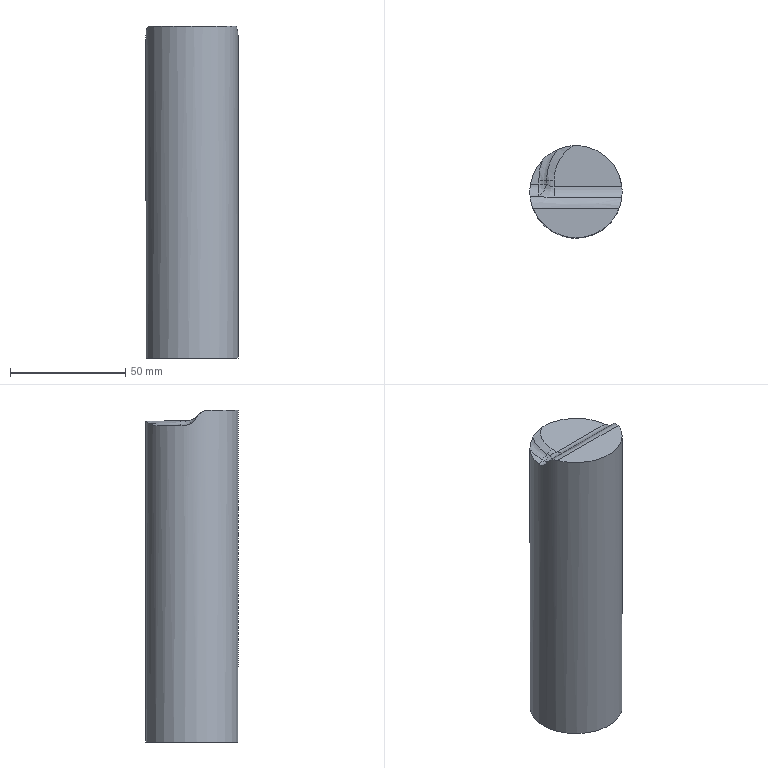Part | NX | features solid 2 | 1 solid | 14 faces | volume 177258 mm3 | spline 12 | cylinder 1 | plane 1 | commonest cylinder face diameters 40 x1
STEP:
#1=CARTESIAN_POINT('',(-644.903,-1.965,-10.409));
#2=VERTEX_POINT('',#1);
#3=CARTESIAN_POINT('',(-643.632,-7.27,-7.114));
#4=VERTEX_POINT('',#3);
#5=CARTESIAN_POINT('',(-644.903,-1.965,-10.409));
#6=CARTESIAN_POINT('',(-644.853,-2.474,-9.401));
#7=CARTESIAN_POINT('',(-644.661,-4.052,-7.717));
#8=CARTESIAN_POINT('',(-644.043,-6.217,-7.123));
#9=CARTESIAN_POINT('',(-643.632,-7.27,-7.114));
#10=B_SPLINE_CURVE_WITH_KNOTS('',3,(#5,#6,#7,#8,#9),.UNSPECIFIED.,.F.,.F.,(4,1,4),(0.,0.003343,0.006685),.UNSPECIFIED.);
#11=EDGE_CURVE('',#2,#4,#10,.T.);
#12=ORIENTED_EDGE('',*,*,#11,.F.);
#13=CARTESIAN_POINT('',(-644.719,3.34,-13.705));
#14=VERTEX_POINT('',#13);
#15=CARTESIAN_POINT('',(-644.719,3.34,-13.705));
#16=CARTESIAN_POINT('',(-645.089,1.157,-13.686));
#17=CARTESIAN_POINT('',(-645.002,-0.9681,-12.383));
#18=CARTESIAN_POINT('',(-644.903,-1.965,-10.409));
#19=B_SPLINE_CURVE_WITH_KNOTS('',3,(#15,#16,#17,#18),.UNSPECIFIED.,.F.,.F.,(4,4),(0.,0.006548),.UNSPECIFIED.);
#20=EDGE_CURVE('',#14,#2,#19,.T.);
#21=ORIENTED_EDGE('',*,*,#20,.F.);
#22=CARTESIAN_POINT('',(-639.509,13.765,-13.794));
#23=VERTEX_POINT('',#22);
#24=CARTESIAN_POINT('',(-639.509,13.765,-13.794));
#25=CARTESIAN_POINT('',(-642.206,10.923,-13.769));
#26=CARTESIAN_POINT('',(-644.056,7.257,-13.738));
#27=CARTESIAN_POINT('',(-644.719,3.34,-13.705));
#28=B_SPLINE_CURVE_WITH_KNOTS('',3,(#24,#25,#26,#27),.UNSPECIFIED.,.F.,.F.,(4,4),(0.04409,0.05584),.UNSPECIFIED.);
#29=EDGE_CURVE('',#23,#14,#28,.T.);
#30=ORIENTED_EDGE('',*,*,#29,.F.);
#31=CARTESIAN_POINT('',(-633.083,18.294,-12.832));
#32=VERTEX_POINT('',#31);
#33=CARTESIAN_POINT('',(-633.083,18.294,-12.832));
#34=CARTESIAN_POINT('',(-635.427,17.258,-13.593));
#35=CARTESIAN_POINT('',(-637.67,15.704,-13.81));
#36=CARTESIAN_POINT('',(-639.509,13.766,-13.794));
#37=B_SPLINE_CURVE_WITH_KNOTS('',3,(#33,#34,#35,#36),.UNSPECIFIED.,.F.,.F.,(4,4),(0.,0.00799),.UNSPECIFIED.);
#38=EDGE_CURVE('',#32,#23,#37,.T.);
#39=ORIENTED_EDGE('',*,*,#38,.F.);
#40=CARTESIAN_POINT('',(-626.243,19.961,-11.846));
#41=VERTEX_POINT('',#40);
#42=CARTESIAN_POINT('',(-626.24,19.962,-11.846));
#43=CARTESIAN_POINT('',(-628.632,19.813,-11.845));
#44=CARTESIAN_POINT('',(-630.98,19.223,-12.15));
#45=CARTESIAN_POINT('',(-633.083,18.294,-12.832));
#46=B_SPLINE_CURVE_WITH_KNOTS('',3,(#42,#43,#44,#45),.UNSPECIFIED.,.F.,.F.,(4,4),(0.,0.007178),.UNSPECIFIED.);
#47=EDGE_CURVE('',#41,#32,#46,.T.);
#48=ORIENTED_EDGE('',*,*,#47,.F.);
#49=CARTESIAN_POINT('',(-605.106,2.059,-11.694));
#50=VERTEX_POINT('',#49);
#51=CARTESIAN_POINT('',(-605.106,2.059,-11.694));
#52=CARTESIAN_POINT('',(-605.371,4.62,-11.715));
#53=CARTESIAN_POINT('',(-606.877,9.562,-11.758));
#54=CARTESIAN_POINT('',(-611.763,15.646,-11.81));
#55=CARTESIAN_POINT('',(-618.55,19.453,-11.842));
#56=CARTESIAN_POINT('',(-623.713,20.119,-11.848));
#57=CARTESIAN_POINT('',(-626.247,19.961,-11.846));
#58=B_SPLINE_CURVE_WITH_KNOTS('',3,(#51,#52,#53,#54,#55,#56,#57),.UNSPECIFIED.,.F.,.F.,(4,1,1,1,4),(0.,0.007614,0.01523,0.02284,0.03046),.UNSPECIFIED.);
#59=EDGE_CURVE('',#50,#41,#58,.T.);
#60=ORIENTED_EDGE('',*,*,#59,.F.);
#61=CARTESIAN_POINT('',(-605.17,-2.605,-9.404));
#62=VERTEX_POINT('',#61);
#63=CARTESIAN_POINT('',(-605.17,-2.605,-9.404));
#64=CARTESIAN_POINT('',(-605.024,-1.49,-10.821));
#65=CARTESIAN_POINT('',(-604.92,0.2592,-11.678));
#66=CARTESIAN_POINT('',(-605.106,2.059,-11.694));
#67=B_SPLINE_CURVE_WITH_KNOTS('',3,(#63,#64,#65,#66),.UNSPECIFIED.,.F.,.F.,(4,4),(0.,0.005391),.UNSPECIFIED.);
#68=EDGE_CURVE('',#62,#50,#67,.T.);
#69=ORIENTED_EDGE('',*,*,#68,.F.);
#70=CARTESIAN_POINT('',(-606.368,-7.27,-7.114));
#71=VERTEX_POINT('',#70);
#72=CARTESIAN_POINT('',(-606.368,-7.27,-7.114));
#73=CARTESIAN_POINT('',(-605.692,-5.537,-7.129));
#74=CARTESIAN_POINT('',(-605.319,-3.738,-7.963));
#75=CARTESIAN_POINT('',(-605.17,-2.605,-9.404));
#76=B_SPLINE_CURVE_WITH_KNOTS('',3,(#72,#73,#74,#75),.UNSPECIFIED.,.F.,.F.,(4,4),(0.,0.005504),.UNSPECIFIED.);
#77=EDGE_CURVE('',#71,#62,#76,.T.);
#78=ORIENTED_EDGE('',*,*,#77,.F.);
#79=CARTESIAN_POINT('',(-643.632,-7.27,-7.114));
#80=CARTESIAN_POINT('',(-642.165,-11.029,-7.082));
#81=CARTESIAN_POINT('',(-636.992,-17.511,-7.026));
#82=CARTESIAN_POINT('',(-624.988,-21.24,-6.994));
#83=CARTESIAN_POINT('',(-615.012,-18.146,-7.021));
#84=CARTESIAN_POINT('',(-609.089,-12.601,-7.068));
#85=CARTESIAN_POINT('',(-607.101,-9.149,-7.098));
#86=CARTESIAN_POINT('',(-606.368,-7.27,-7.114));
#87=B_SPLINE_CURVE_WITH_KNOTS('',3,(#79,#80,#81,#82,#83,#84,#85,#86),.UNSPECIFIED.,.F.,.F.,(4,1,1,1,1,4),(0.,0.01194,0.02387,0.03581,0.04177,0.04774),.UNSPECIFIED.);
#88=EDGE_CURVE('',#4,#71,#87,.T.);
#89=ORIENTED_EDGE('',*,*,#88,.F.);
#90=EDGE_LOOP('',(#12,#21,#30,#39,#48,#60,#69,#78,#89));
#91=FACE_BOUND('',#90,.T.);
#92=CARTESIAN_POINT('',(-605.,0.,-151.));
#93=VERTEX_POINT('',#92);
#94=CARTESIAN_POINT('',(-625.,0.,-151.));
#95=DIRECTION('',(0.,0.,1.));
#96=DIRECTION('',(1.,0.,0.));
#97=AXIS2_PLACEMENT_3D('',#94,#95,#96);
#98=CIRCLE('',#97,20.);
#99=EDGE_CURVE('',#93,#93,#98,.F.);
#100=ORIENTED_EDGE('',*,*,#99,.F.);
#101=EDGE_LOOP('',(#100));
#102=FACE_BOUND('',#101,.T.);
#103=CARTESIAN_POINT('',(-625.,0.,40.));
#104=DIRECTION('',(0.,0.,-1.));
#105=DIRECTION('',(-1.,0.,0.));
#106=AXIS2_PLACEMENT_3D('',#103,#104,#105);
#107=CYLINDRICAL_SURFACE('',#106,20.);
#108=ADVANCED_FACE('',(#91,#102),#107,.T.);
#109=ORIENTED_EDGE('',*,*,#99,.T.);
#110=EDGE_LOOP('',(#109));
#111=FACE_BOUND('',#110,.T.);
#112=CARTESIAN_POINT('',(-615.,0.,-151.));
#113=DIRECTION('',(0.,0.,1.));
#114=DIRECTION('',(1.,0.,0.));
#115=AXIS2_PLACEMENT_3D('',#112,#113,#114);
#116=PLANE('',#115);
#117=ADVANCED_FACE('',(#111),#116,.F.);
#118=ORIENTED_EDGE('',*,*,#29,.T.);
#119=CARTESIAN_POINT('',(-641.148,3.34,-13.705));
#120=VERTEX_POINT('',#119);
#121=CARTESIAN_POINT('',(-641.148,3.34,-13.705));
#122=CARTESIAN_POINT('',(-647.,3.34,-13.705));
#123=(BOUNDED_CURVE()B_SPLINE_CURVE(1,(#121,#122),.UNSPECIFIED.,.F.,.F.)B_SPLINE_CURVE_WITH_KNOTS((2,2),(0.,1.),.PIECEWISE_BEZIER_KNOTS.)CURVE()GEOMETRIC_REPRESENTATION_ITEM()RATIONAL_B_SPLINE_CURVE((1.,1.))REPRESENTATION_ITEM(''));
#124=EDGE_CURVE('',#14,#120,#123,.F.);
#125=ORIENTED_EDGE('',*,*,#124,.T.);
#126=CARTESIAN_POINT('',(-641.148,4.988,-13.719));
#127=VERTEX_POINT('',#126);
#128=CARTESIAN_POINT('',(-641.148,3.34,-13.705));
#129=CARTESIAN_POINT('',(-641.148,3.889,-13.709));
#130=CARTESIAN_POINT('',(-641.148,4.438,-13.714));
#131=CARTESIAN_POINT('',(-641.148,4.988,-13.719));
#132=B_SPLINE_CURVE_WITH_KNOTS('',3,(#128,#129,#130,#131),.UNSPECIFIED.,.F.,.F.,(4,4),(0.,1.),.UNSPECIFIED.);
#133=EDGE_CURVE('',#120,#127,#132,.T.);
#134=ORIENTED_EDGE('',*,*,#133,.T.);
#135=CARTESIAN_POINT('',(-641.148,4.988,-13.719));
#136=CARTESIAN_POINT('',(-641.148,8.023,-13.744));
#137=CARTESIAN_POINT('',(-640.602,10.949,-13.769));
#138=CARTESIAN_POINT('',(-639.509,13.765,-13.794));
#139=B_SPLINE_CURVE_WITH_KNOTS('',3,(#135,#136,#137,#138),.UNSPECIFIED.,.F.,.F.,(4,4),(0.,0.2363),.UNSPECIFIED.);
#140=EDGE_CURVE('',#127,#23,#139,.T.);
#141=ORIENTED_EDGE('',*,*,#140,.T.);
#142=EDGE_LOOP('',(#118,#125,#134,#141));
#143=FACE_BOUND('',#142,.T.);
#144=CARTESIAN_POINT('',(-639.478,13.828,-13.794));
#145=CARTESIAN_POINT('',(-644.75,13.828,-13.794));
#146=CARTESIAN_POINT('',(-639.478,3.34,-13.705));
#147=CARTESIAN_POINT('',(-644.75,3.34,-13.705));
#148=B_SPLINE_SURFACE_WITH_KNOTS('',1,1,((#144,#145),(#146,#147)),.PLANE_SURF.,.F.,.F.,.F.,(2,2),(2,2),(0.7723,1.),(0.9535,0.9861),.PIECEWISE_BEZIER_KNOTS.);
#149=ADVANCED_FACE('',(#143),#148,.F.);
#150=ORIENTED_EDGE('',*,*,#38,.T.);
#151=ORIENTED_EDGE('',*,*,#140,.F.);
#152=CARTESIAN_POINT('',(-637.831,4.996,-12.719));
#153=VERTEX_POINT('',#152);
#154=CARTESIAN_POINT('',(-637.831,4.996,-12.719));
#155=CARTESIAN_POINT('',(-638.807,4.991,-13.366));
#156=CARTESIAN_POINT('',(-639.977,4.988,-13.719));
#157=CARTESIAN_POINT('',(-641.148,4.988,-13.719));
#158=B_SPLINE_CURVE_WITH_KNOTS('',3,(#154,#155,#156,#157),.UNSPECIFIED.,.F.,.F.,(4,4),(0.,1.),.UNSPECIFIED.);
#159=EDGE_CURVE('',#127,#153,#158,.F.);
#160=ORIENTED_EDGE('',*,*,#159,.T.);
#161=CARTESIAN_POINT('',(-633.083,18.294,-12.832));
#162=CARTESIAN_POINT('',(-636.122,14.585,-12.8));
#163=CARTESIAN_POINT('',(-637.831,9.804,-12.76));
#164=CARTESIAN_POINT('',(-637.831,4.996,-12.719));
#165=B_SPLINE_CURVE_WITH_KNOTS('',3,(#161,#162,#163,#164),.UNSPECIFIED.,.F.,.F.,(4,4),(0.5612,1.),.UNSPECIFIED.);
#166=EDGE_CURVE('',#153,#32,#165,.F.);
#167=ORIENTED_EDGE('',*,*,#166,.T.);
#168=EDGE_LOOP('',(#150,#151,#160,#167));
#169=FACE_BOUND('',#168,.T.);
#170=CARTESIAN_POINT('',(-641.148,4.988,-13.719));
#171=CARTESIAN_POINT('',(-640.445,4.988,-13.719));
#172=CARTESIAN_POINT('',(-639.742,4.988,-13.616));
#173=CARTESIAN_POINT('',(-639.06,4.99,-13.41));
#174=CARTESIAN_POINT('',(-638.417,4.993,-13.107));
#175=CARTESIAN_POINT('',(-637.831,4.996,-12.719));
#176=CARTESIAN_POINT('',(-641.148,5.525,-13.723));
#177=CARTESIAN_POINT('',(-640.445,5.509,-13.723));
#178=CARTESIAN_POINT('',(-639.742,5.495,-13.62));
#179=CARTESIAN_POINT('',(-639.06,5.481,-13.414));
#180=CARTESIAN_POINT('',(-638.417,5.47,-13.111));
#181=CARTESIAN_POINT('',(-637.831,5.46,-12.723));
#182=CARTESIAN_POINT('',(-641.133,6.068,-13.728));
#183=CARTESIAN_POINT('',(-640.431,6.036,-13.728));
#184=CARTESIAN_POINT('',(-639.728,6.006,-13.624));
#185=CARTESIAN_POINT('',(-639.046,5.977,-13.418));
#186=CARTESIAN_POINT('',(-638.404,5.951,-13.115));
#187=CARTESIAN_POINT('',(-637.818,5.929,-12.727));
#188=CARTESIAN_POINT('',(-641.103,6.599,-13.732));
#189=CARTESIAN_POINT('',(-640.402,6.552,-13.732));
#190=CARTESIAN_POINT('',(-639.7,6.507,-13.629));
#191=CARTESIAN_POINT('',(-639.019,6.463,-13.422));
#192=CARTESIAN_POINT('',(-638.377,6.423,-13.119));
#193=CARTESIAN_POINT('',(-637.793,6.388,-12.731));
#194=CARTESIAN_POINT('',(-641.015,7.671,-13.741));
#195=CARTESIAN_POINT('',(-640.316,7.594,-13.741));
#196=CARTESIAN_POINT('',(-639.617,7.517,-13.637));
#197=CARTESIAN_POINT('',(-638.938,7.444,-13.431));
#198=CARTESIAN_POINT('',(-638.299,7.375,-13.127));
#199=CARTESIAN_POINT('',(-637.716,7.314,-12.738));
#200=CARTESIAN_POINT('',(-640.867,8.733,-13.751));
#201=CARTESIAN_POINT('',(-640.172,8.625,-13.75));
#202=CARTESIAN_POINT('',(-639.477,8.517,-13.646));
#203=CARTESIAN_POINT('',(-638.803,8.414,-13.439));
#204=CARTESIAN_POINT('',(-638.167,8.318,-13.135));
#205=CARTESIAN_POINT('',(-637.589,8.231,-12.746));
#206=CARTESIAN_POINT('',(-640.778,9.264,-13.755));
#207=CARTESIAN_POINT('',(-640.086,9.14,-13.754));
#208=CARTESIAN_POINT('',(-639.394,9.018,-13.65));
#209=CARTESIAN_POINT('',(-638.722,8.899,-13.443));
#210=CARTESIAN_POINT('',(-638.089,8.789,-13.14));
#211=CARTESIAN_POINT('',(-637.512,8.689,-12.75));
#212=CARTESIAN_POINT('',(-640.469,10.845,-13.769));
#213=CARTESIAN_POINT('',(-639.786,10.675,-13.767));
#214=CARTESIAN_POINT('',(-639.103,10.507,-13.663));
#215=CARTESIAN_POINT('',(-638.439,10.344,-13.456));
#216=CARTESIAN_POINT('',(-637.814,10.192,-13.151));
#217=CARTESIAN_POINT('',(-637.245,10.055,-12.762));
#218=CARTESIAN_POINT('',(-640.03,12.396,-13.782));
#219=CARTESIAN_POINT('',(-639.359,12.182,-13.78));
#220=CARTESIAN_POINT('',(-638.689,11.969,-13.675));
#221=CARTESIAN_POINT('',(-638.037,11.763,-13.468));
#222=CARTESIAN_POINT('',(-637.424,11.57,-13.163));
#223=CARTESIAN_POINT('',(-636.866,11.395,-12.773));
#224=CARTESIAN_POINT('',(-639.68,13.413,-13.791));
#225=CARTESIAN_POINT('',(-639.02,13.17,-13.788));
#226=CARTESIAN_POINT('',(-638.359,12.927,-13.683));
#227=CARTESIAN_POINT('',(-637.718,12.692,-13.476));
#228=CARTESIAN_POINT('',(-637.114,12.472,-13.171));
#229=CARTESIAN_POINT('',(-636.564,12.273,-12.781));
#230=CARTESIAN_POINT('',(-638.819,15.53,-13.809));
#231=CARTESIAN_POINT('',(-638.183,15.225,-13.806));
#232=CARTESIAN_POINT('',(-637.548,14.921,-13.7));
#233=CARTESIAN_POINT('',(-636.931,14.627,-13.492));
#234=CARTESIAN_POINT('',(-636.35,14.351,-13.187));
#235=CARTESIAN_POINT('',(-635.82,14.101,-12.796));
#236=CARTESIAN_POINT('',(-637.715,17.532,-13.826));
#237=CARTESIAN_POINT('',(-637.112,17.169,-13.823));
#238=CARTESIAN_POINT('',(-636.508,16.807,-13.717));
#239=CARTESIAN_POINT('',(-635.922,16.457,-13.508));
#240=CARTESIAN_POINT('',(-635.37,16.128,-13.202));
#241=CARTESIAN_POINT('',(-634.867,15.829,-12.811));
#242=CARTESIAN_POINT('',(-637.066,18.554,-13.834));
#243=CARTESIAN_POINT('',(-636.481,18.162,-13.831));
#244=CARTESIAN_POINT('',(-635.896,17.771,-13.725));
#245=CARTESIAN_POINT('',(-635.328,17.391,-13.516));
#246=CARTESIAN_POINT('',(-634.794,17.035,-13.21));
#247=CARTESIAN_POINT('',(-634.306,16.712,-12.819));
#248=CARTESIAN_POINT('',(-636.354,19.534,-13.843));
#249=CARTESIAN_POINT('',(-635.79,19.113,-13.839));
#250=CARTESIAN_POINT('',(-635.226,18.693,-13.733));
#251=CARTESIAN_POINT('',(-634.678,18.286,-13.523));
#252=CARTESIAN_POINT('',(-634.162,17.904,-13.217));
#253=CARTESIAN_POINT('',(-633.692,17.557,-12.826));
#254=CARTESIAN_POINT('',(-635.584,20.465,-13.851));
#255=CARTESIAN_POINT('',(-635.042,20.017,-13.847));
#256=CARTESIAN_POINT('',(-634.501,19.57,-13.74));
#257=CARTESIAN_POINT('',(-633.974,19.137,-13.531));
#258=CARTESIAN_POINT('',(-633.479,18.731,-13.224));
#259=CARTESIAN_POINT('',(-633.028,18.361,-12.833));
#260=B_SPLINE_SURFACE_WITH_KNOTS('',5,5,((#170,#171,#172,#173,#174,#175),(#176,#177,#178,#179,#180,#181),(#182,#183,#184,#185,#186,#187),(#188,#189,#190,#191,#192,#193),(#194,#195,#196,#197,#198,#199),(#200,#201,#202,#203,#204,#205),(#206,#207,#208,#209,#210,#211),(#212,#213,#214,#215,#216,#217),(#218,#219,#220,#221,#222,#223),(#224,#225,#226,#227,#228,#229),(#230,#231,#232,#233,#234,#235),(#236,#237,#238,#239,#240,#241),(#242,#243,#244,#245,#246,#247),(#248,#249,#250,#251,#252,#253),(#254,#255,#256,#257,#258,#259)),.UNSPECIFIED.,.F.,.F.,.F.,(6,3,3,3,6),(6,6),(0.,0.0706,0.1412,0.2824,0.4414),(0.,1.),.UNSPECIFIED.);
#261=ADVANCED_FACE('',(#169),#260,.F.);
#262=CARTESIAN_POINT('',(-637.831,3.349,-12.705));
#263=VERTEX_POINT('',#262);
#264=CARTESIAN_POINT('',(-637.831,3.349,-12.705));
#265=CARTESIAN_POINT('',(-638.794,3.343,-13.343));
#266=CARTESIAN_POINT('',(-639.993,3.34,-13.705));
#267=CARTESIAN_POINT('',(-641.148,3.34,-13.705));
#268=B_SPLINE_CURVE_WITH_KNOTS('',3,(#264,#265,#266,#267),.UNSPECIFIED.,.F.,.F.,(4,4),(0.,1.),.UNSPECIFIED.);
#269=EDGE_CURVE('',#120,#263,#268,.F.);
#270=ORIENTED_EDGE('',*,*,#269,.T.);
#271=CARTESIAN_POINT('',(-637.831,4.996,-12.719));
#272=CARTESIAN_POINT('',(-637.831,4.447,-12.714));
#273=CARTESIAN_POINT('',(-637.831,3.898,-12.709));
#274=CARTESIAN_POINT('',(-637.831,3.349,-12.705));
#275=B_SPLINE_CURVE_WITH_KNOTS('',3,(#271,#272,#273,#274),.UNSPECIFIED.,.F.,.F.,(4,4),(0.,1.),.UNSPECIFIED.);
#276=EDGE_CURVE('',#153,#263,#275,.T.);
#277=ORIENTED_EDGE('',*,*,#276,.F.);
#278=ORIENTED_EDGE('',*,*,#159,.F.);
#279=ORIENTED_EDGE('',*,*,#133,.F.);
#280=EDGE_LOOP('',(#270,#277,#278,#279));
#281=FACE_BOUND('',#280,.T.);
#282=CARTESIAN_POINT('',(-637.831,3.349,-12.705));
#283=CARTESIAN_POINT('',(-637.831,4.996,-12.719));
#284=CARTESIAN_POINT('',(-638.822,3.343,-13.361));
#285=CARTESIAN_POINT('',(-638.822,4.99,-13.376));
#286=CARTESIAN_POINT('',(-639.96,3.34,-13.705));
#287=CARTESIAN_POINT('',(-639.96,4.988,-13.719));
#288=CARTESIAN_POINT('',(-641.148,3.34,-13.705));
#289=CARTESIAN_POINT('',(-641.148,4.988,-13.719));
#290=(BOUNDED_SURFACE()B_SPLINE_SURFACE(3,1,((#282,#283),(#284,#285),(#286,#287),(#288,#289)),.CYLINDRICAL_SURF.,.F.,.F.,.F.)B_SPLINE_SURFACE_WITH_KNOTS((4,4),(2,2),(0.,1.),(0.,1.),.PIECEWISE_BEZIER_KNOTS.)GEOMETRIC_REPRESENTATION_ITEM()RATIONAL_B_SPLINE_SURFACE(((1.,1.),(0.9716,0.9716),(0.9716,0.9716),(1.,1.)))REPRESENTATION_ITEM('')SURFACE());
#291=ADVANCED_FACE('',(#281),#290,.F.);
#292=ORIENTED_EDGE('',*,*,#20,.T.);
#293=CARTESIAN_POINT('',(-641.148,-1.965,-10.409));
#294=VERTEX_POINT('',#293);
#295=CARTESIAN_POINT('',(-641.148,-1.965,-10.409));
#296=CARTESIAN_POINT('',(-642.4,-1.965,-10.409));
#297=CARTESIAN_POINT('',(-643.651,-1.965,-10.409));
#298=CARTESIAN_POINT('',(-644.903,-1.965,-10.409));
#299=B_SPLINE_CURVE_WITH_KNOTS('',3,(#295,#296,#297,#298),.UNSPECIFIED.,.F.,.F.,(4,4),(0.,0.6417),.UNSPECIFIED.);
#300=EDGE_CURVE('',#294,#2,#299,.T.);
#301=ORIENTED_EDGE('',*,*,#300,.F.);
#302=CARTESIAN_POINT('',(-641.148,3.34,-13.705));
#303=CARTESIAN_POINT('',(-641.148,2.299,-13.696));
#304=CARTESIAN_POINT('',(-641.148,0.04839,-13.086));
#305=CARTESIAN_POINT('',(-641.148,-1.496,-11.338));
#306=CARTESIAN_POINT('',(-641.148,-1.965,-10.409));
#307=B_SPLINE_CURVE_WITH_KNOTS('',3,(#302,#303,#304,#305,#306),.UNSPECIFIED.,.F.,.F.,(4,1,4),(0.,0.5,1.),.UNSPECIFIED.);
#308=EDGE_CURVE('',#120,#294,#307,.T.);
#309=ORIENTED_EDGE('',*,*,#308,.F.);
#310=ORIENTED_EDGE('',*,*,#124,.F.);
#311=EDGE_LOOP('',(#292,#301,#309,#310));
#312=FACE_BOUND('',#311,.T.);
#313=CARTESIAN_POINT('',(-641.148,3.34,-13.705));
#314=CARTESIAN_POINT('',(-645.028,3.34,-13.705));
#315=CARTESIAN_POINT('',(-641.148,1.034,-13.685));
#316=CARTESIAN_POINT('',(-645.028,1.034,-13.685));
#317=CARTESIAN_POINT('',(-641.148,-0.9252,-12.468));
#318=CARTESIAN_POINT('',(-645.028,-0.9252,-12.468));
#319=CARTESIAN_POINT('',(-641.148,-1.965,-10.409));
#320=CARTESIAN_POINT('',(-645.028,-1.965,-10.409));
#321=(BOUNDED_SURFACE()B_SPLINE_SURFACE(3,1,((#313,#314),(#315,#316),(#317,#318),(#319,#320)),.CYLINDRICAL_SURF.,.F.,.F.,.F.)B_SPLINE_SURFACE_WITH_KNOTS((4,4),(2,2),(0.,1.),(0.,0.6631),.PIECEWISE_BEZIER_KNOTS.)GEOMETRIC_REPRESENTATION_ITEM()RATIONAL_B_SPLINE_SURFACE(((1.,1.),(0.9026,0.9026),(0.9026,0.9026),(1.,1.)))REPRESENTATION_ITEM('')SURFACE());
#322=ADVANCED_FACE('',(#312),#321,.F.);
#323=ORIENTED_EDGE('',*,*,#47,.T.);
#324=ORIENTED_EDGE('',*,*,#166,.F.);
#325=CARTESIAN_POINT('',(-634.515,5.005,-11.719));
#326=VERTEX_POINT('',#325);
#327=CARTESIAN_POINT('',(-634.515,5.005,-11.719));
#328=CARTESIAN_POINT('',(-635.686,5.005,-11.719));
#329=CARTESIAN_POINT('',(-636.855,5.002,-12.071));
#330=CARTESIAN_POINT('',(-637.831,4.996,-12.719));
#331=B_SPLINE_CURVE_WITH_KNOTS('',3,(#327,#328,#329,#330),.UNSPECIFIED.,.F.,.F.,(4,4),(0.,1.),.UNSPECIFIED.);
#332=EDGE_CURVE('',#326,#153,#331,.T.);
#333=ORIENTED_EDGE('',*,*,#332,.F.);
#334=CARTESIAN_POINT('',(-626.243,19.96,-11.846));
#335=CARTESIAN_POINT('',(-628.759,18.388,-11.833));
#336=CARTESIAN_POINT('',(-632.976,13.938,-11.795));
#337=CARTESIAN_POINT('',(-634.515,7.986,-11.744));
#338=CARTESIAN_POINT('',(-634.515,5.005,-11.719));
#339=B_SPLINE_CURVE_WITH_KNOTS('',3,(#334,#335,#336,#337,#338),.UNSPECIFIED.,.F.,.F.,(4,1,4),(0.3537,0.6768,1.),.UNSPECIFIED.);
#340=EDGE_CURVE('',#326,#41,#339,.F.);
#341=ORIENTED_EDGE('',*,*,#340,.T.);
#342=EDGE_LOOP('',(#323,#324,#333,#341));
#343=FACE_BOUND('',#342,.T.);
#344=CARTESIAN_POINT('',(-626.149,20.018,-11.847));
#345=CARTESIAN_POINT('',(-626.518,20.616,-11.852));
#346=CARTESIAN_POINT('',(-626.886,21.214,-11.96));
#347=CARTESIAN_POINT('',(-627.244,21.793,-12.171));
#348=CARTESIAN_POINT('',(-627.581,22.338,-12.478));
#349=CARTESIAN_POINT('',(-627.888,22.833,-12.871));
#350=CARTESIAN_POINT('',(-626.484,19.812,-11.845));
#351=CARTESIAN_POINT('',(-626.866,20.402,-11.85));
#352=CARTESIAN_POINT('',(-627.248,20.991,-11.958));
#353=CARTESIAN_POINT('',(-627.619,21.563,-12.169));
#354=CARTESIAN_POINT('',(-627.968,22.1,-12.476));
#355=CARTESIAN_POINT('',(-628.286,22.588,-12.869));
#356=CARTESIAN_POINT('',(-626.812,19.597,-11.843));
#357=CARTESIAN_POINT('',(-627.207,20.178,-11.848));
#358=CARTESIAN_POINT('',(-627.602,20.759,-11.956));
#359=CARTESIAN_POINT('',(-627.986,21.322,-12.167));
#360=CARTESIAN_POINT('',(-628.348,21.851,-12.474));
#361=CARTESIAN_POINT('',(-628.677,22.332,-12.867));
#362=CARTESIAN_POINT('',(-627.135,19.372,-11.841));
#363=CARTESIAN_POINT('',(-627.543,19.945,-11.846));
#364=CARTESIAN_POINT('',(-627.951,20.516,-11.954));
#365=CARTESIAN_POINT('',(-628.347,21.071,-12.165));
#366=CARTESIAN_POINT('',(-628.72,21.591,-12.472));
#367=CARTESIAN_POINT('',(-629.06,22.065,-12.864));
#368=CARTESIAN_POINT('',(-630.018,17.243,-11.823));
#369=CARTESIAN_POINT('',(-630.542,17.73,-11.827));
#370=CARTESIAN_POINT('',(-631.066,18.216,-11.934));
#371=CARTESIAN_POINT('',(-631.574,18.687,-12.144));
#372=CARTESIAN_POINT('',(-632.053,19.13,-12.451));
#373=CARTESIAN_POINT('',(-632.49,19.533,-12.843));
#374=CARTESIAN_POINT('',(-632.34,14.391,-11.799));
#375=CARTESIAN_POINT('',(-632.956,14.764,-11.802));
#376=CARTESIAN_POINT('',(-633.572,15.136,-11.908));
#377=CARTESIAN_POINT('',(-634.171,15.496,-12.117));
#378=CARTESIAN_POINT('',(-634.735,15.835,-12.423));
#379=CARTESIAN_POINT('',(-635.249,16.142,-12.814));
#380=CARTESIAN_POINT('',(-633.79,11.411,-11.773));
#381=CARTESIAN_POINT('',(-634.464,11.666,-11.776));
#382=CARTESIAN_POINT('',(-635.138,11.92,-11.881));
#383=CARTESIAN_POINT('',(-635.793,12.166,-12.089));
#384=CARTESIAN_POINT('',(-636.409,12.396,-12.393));
#385=CARTESIAN_POINT('',(-636.971,12.605,-12.784));
#386=CARTESIAN_POINT('',(-634.515,8.21,-11.746));
#387=CARTESIAN_POINT('',(-635.218,8.337,-11.747));
#388=CARTESIAN_POINT('',(-635.92,8.463,-11.851));
#389=CARTESIAN_POINT('',(-636.603,8.584,-12.058));
#390=CARTESIAN_POINT('',(-637.246,8.698,-12.362));
#391=CARTESIAN_POINT('',(-637.831,8.8,-12.751));
#392=CARTESIAN_POINT('',(-634.515,5.005,-11.719));
#393=CARTESIAN_POINT('',(-635.218,5.005,-11.719));
#394=CARTESIAN_POINT('',(-635.92,5.004,-11.822));
#395=CARTESIAN_POINT('',(-636.603,5.002,-12.027));
#396=CARTESIAN_POINT('',(-637.246,4.999,-12.33));
#397=CARTESIAN_POINT('',(-637.831,4.996,-12.719));
#398=B_SPLINE_SURFACE_WITH_KNOTS('',5,5,((#344,#345,#346,#347,#348,#349),(#350,#351,#352,#353,#354,#355),(#356,#357,#358,#359,#360,#361),(#362,#363,#364,#365,#366,#367),(#368,#369,#370,#371,#372,#373),(#374,#375,#376,#377,#378,#379),(#380,#381,#382,#383,#384,#385),(#386,#387,#388,#389,#390,#391),(#392,#393,#394,#395,#396,#397)),.UNSPECIFIED.,.F.,.F.,.F.,(6,3,6),(6,6),(0.3497,0.421,1.),(0.,0.994),.UNSPECIFIED.);
#399=ADVANCED_FACE('',(#343),#398,.F.);
#400=CARTESIAN_POINT('',(-634.515,2.059,-11.694));
#401=VERTEX_POINT('',#400);
#402=CARTESIAN_POINT('',(-634.515,2.059,-11.694));
#403=CARTESIAN_POINT('',(-634.515,3.041,-11.702));
#404=CARTESIAN_POINT('',(-634.515,4.023,-11.71));
#405=CARTESIAN_POINT('',(-634.515,5.005,-11.719));
#406=B_SPLINE_CURVE_WITH_KNOTS('',3,(#402,#403,#404,#405),.UNSPECIFIED.,.F.,.F.,(4,4),(0.,1.),.UNSPECIFIED.);
#407=EDGE_CURVE('',#401,#326,#406,.T.);
#408=ORIENTED_EDGE('',*,*,#407,.T.);
#409=ORIENTED_EDGE('',*,*,#332,.T.);
#410=ORIENTED_EDGE('',*,*,#276,.T.);
#411=CARTESIAN_POINT('',(-637.831,3.349,-12.705));
#412=CARTESIAN_POINT('',(-637.491,3.118,-12.477));
#413=CARTESIAN_POINT('',(-637.023,2.834,-12.235));
#414=CARTESIAN_POINT('',(-636.498,2.559,-12.033));
#415=CARTESIAN_POINT('',(-636.275,2.45,-11.956));
#416=CARTESIAN_POINT('',(-635.774,2.258,-11.821));
#417=CARTESIAN_POINT('',(-635.212,2.11,-11.724));
#418=CARTESIAN_POINT('',(-634.784,2.059,-11.694));
#419=CARTESIAN_POINT('',(-634.515,2.059,-11.694));
#420=B_SPLINE_CURVE_WITH_KNOTS('',3,(#411,#412,#413,#414,#415,#416,#417,#418,#419),.UNSPECIFIED.,.F.,.F.,(4,1,1,1,1,1,4),(0.,0.25,0.375,0.5,0.625,0.75,1.),.UNSPECIFIED.);
#421=EDGE_CURVE('',#263,#401,#420,.T.);
#422=ORIENTED_EDGE('',*,*,#421,.T.);
#423=EDGE_LOOP('',(#408,#409,#410,#422));
#424=FACE_BOUND('',#423,.T.);
#425=CARTESIAN_POINT('',(-634.515,5.005,-11.719));
#426=CARTESIAN_POINT('',(-634.515,2.042,-11.693));
#427=CARTESIAN_POINT('',(-635.703,5.005,-11.719));
#428=CARTESIAN_POINT('',(-635.703,2.042,-11.693));
#429=CARTESIAN_POINT('',(-636.841,5.002,-12.062));
#430=CARTESIAN_POINT('',(-636.841,2.039,-12.036));
#431=CARTESIAN_POINT('',(-637.831,4.996,-12.719));
#432=CARTESIAN_POINT('',(-637.831,2.033,-12.693));
#433=(BOUNDED_SURFACE()B_SPLINE_SURFACE(3,1,((#425,#426),(#427,#428),(#429,#430),(#431,#432)),.CYLINDRICAL_SURF.,.F.,.F.,.F.)B_SPLINE_SURFACE_WITH_KNOTS((4,4),(2,2),(0.,1.),(0.08333,0.9167),.PIECEWISE_BEZIER_KNOTS.)GEOMETRIC_REPRESENTATION_ITEM()RATIONAL_B_SPLINE_SURFACE(((1.,1.),(0.9716,0.9716),(0.9716,0.9716),(1.,1.)))REPRESENTATION_ITEM('')SURFACE());
#434=ADVANCED_FACE('',(#424),#433,.T.);
#435=ORIENTED_EDGE('',*,*,#269,.F.);
#436=ORIENTED_EDGE('',*,*,#308,.T.);
#437=CARTESIAN_POINT('',(-637.831,3.349,-12.705));
#438=CARTESIAN_POINT('',(-637.945,2.867,-12.776));
#439=CARTESIAN_POINT('',(-638.183,2.089,-12.821));
#440=CARTESIAN_POINT('',(-638.623,1.1,-12.657));
#441=CARTESIAN_POINT('',(-638.898,0.5681,-12.509));
#442=CARTESIAN_POINT('',(-639.187,0.08387,-12.317));
#443=CARTESIAN_POINT('',(-639.272,-0.04024,-12.256));
#444=CARTESIAN_POINT('',(-639.51,-0.3857,-12.082));
#445=CARTESIAN_POINT('',(-640.003,-1.019,-11.678));
#446=CARTESIAN_POINT('',(-640.644,-1.662,-11.01));
#447=CARTESIAN_POINT('',(-641.148,-1.965,-10.409));
#448=B_SPLINE_CURVE_WITH_KNOTS('',3,(#437,#438,#439,#440,#441,#442,#443,#444,#445,#446,#447),.UNSPECIFIED.,.F.,.F.,(4,1,1,1,1,1,1,1,4),(0.,0.25,0.375,0.4375,0.5,0.5625,0.625,0.75,1.),.UNSPECIFIED.);
#449=EDGE_CURVE('',#294,#263,#448,.F.);
#450=ORIENTED_EDGE('',*,*,#449,.T.);
#451=EDGE_LOOP('',(#435,#436,#450));
#452=FACE_BOUND('',#451,.T.);
#453=CARTESIAN_POINT('',(-641.148,3.34,-13.705));
#454=CARTESIAN_POINT('',(-641.148,1.018,-13.685));
#455=CARTESIAN_POINT('',(-641.148,-0.9487,-12.453));
#456=CARTESIAN_POINT('',(-641.148,-1.982,-10.376));
#457=CARTESIAN_POINT('',(-639.952,3.34,-13.705));
#458=CARTESIAN_POINT('',(-639.952,1.018,-13.685));
#459=CARTESIAN_POINT('',(-639.952,-0.9487,-12.453));
#460=CARTESIAN_POINT('',(-639.952,-1.982,-10.376));
#461=CARTESIAN_POINT('',(-638.808,3.343,-13.357));
#462=CARTESIAN_POINT('',(-638.808,1.156,-13.339));
#463=CARTESIAN_POINT('',(-638.808,-0.6976,-12.178));
#464=CARTESIAN_POINT('',(-638.808,-1.671,-10.221));
#465=CARTESIAN_POINT('',(-637.814,3.349,-12.693));
#466=CARTESIAN_POINT('',(-637.814,1.418,-12.677));
#467=CARTESIAN_POINT('',(-637.814,-0.2171,-11.653));
#468=CARTESIAN_POINT('',(-637.814,-1.076,-9.925));
#469=(BOUNDED_SURFACE()B_SPLINE_SURFACE(3,3,((#453,#454,#455,#456),(#457,#458,#459,#460),(#461,#462,#463,#464),(#465,#466,#467,#468)),.SPHERICAL_SURF.,.F.,.F.,.F.)B_SPLINE_SURFACE_WITH_KNOTS((4,4),(4,4),(0.,0.9999),(0.08628,0.9189),.PIECEWISE_BEZIER_KNOTS.)GEOMETRIC_REPRESENTATION_ITEM()RATIONAL_B_SPLINE_SURFACE(((0.9675,0.8727,0.8733,0.9692),(0.9397,0.8476,0.8482,0.9414),(0.9397,0.8476,0.8482,0.9414),(0.9675,0.8727,0.8733,0.9692)))REPRESENTATION_ITEM('')SURFACE());
#470=ADVANCED_FACE('',(#452),#469,.F.);
#471=ORIENTED_EDGE('',*,*,#59,.T.);
#472=ORIENTED_EDGE('',*,*,#340,.F.);
#473=ORIENTED_EDGE('',*,*,#407,.F.);
#474=CARTESIAN_POINT('',(-605.106,2.059,-11.694));
#475=CARTESIAN_POINT('',(-614.909,2.059,-11.694));
#476=CARTESIAN_POINT('',(-624.712,2.059,-11.694));
#477=CARTESIAN_POINT('',(-634.515,2.059,-11.694));
#478=B_SPLINE_CURVE_WITH_KNOTS('',3,(#474,#475,#476,#477),.UNSPECIFIED.,.F.,.F.,(4,4),(0.5973,1.),.UNSPECIFIED.);
#479=EDGE_CURVE('',#401,#50,#478,.F.);
#480=ORIENTED_EDGE('',*,*,#479,.T.);
#481=EDGE_LOOP('',(#471,#472,#473,#480));
#482=FACE_BOUND('',#481,.T.);
#483=CARTESIAN_POINT('',(-604.93,20.144,-11.848));
#484=CARTESIAN_POINT('',(-634.515,20.144,-11.848));
#485=CARTESIAN_POINT('',(-604.93,2.059,-11.694));
#486=CARTESIAN_POINT('',(-634.515,2.059,-11.694));
#487=B_SPLINE_SURFACE_WITH_KNOTS('',1,1,((#483,#484),(#485,#486)),.PLANE_SURF.,.F.,.F.,.F.,(2,2),(2,2),(0.12,1.),(0.5949,1.),.PIECEWISE_BEZIER_KNOTS.);
#488=ADVANCED_FACE('',(#482),#487,.F.);
#489=CARTESIAN_POINT('',(-634.515,-2.605,-9.404));
#490=VERTEX_POINT('',#489);
#491=CARTESIAN_POINT('',(-634.515,-2.605,-9.404));
#492=CARTESIAN_POINT('',(-636.83,-2.605,-9.404));
#493=CARTESIAN_POINT('',(-639.111,-2.307,-9.731));
#494=CARTESIAN_POINT('',(-641.148,-1.965,-10.409));
#495=B_SPLINE_CURVE_WITH_KNOTS('',3,(#491,#492,#493,#494),.UNSPECIFIED.,.F.,.F.,(4,4),(0.,1.),.UNSPECIFIED.);
#496=EDGE_CURVE('',#490,#294,#495,.T.);
#497=ORIENTED_EDGE('',*,*,#496,.F.);
#498=CARTESIAN_POINT('',(-634.515,2.059,-11.694));
#499=CARTESIAN_POINT('',(-634.515,0.268,-11.678));
#500=CARTESIAN_POINT('',(-634.515,-1.498,-10.811));
#501=CARTESIAN_POINT('',(-634.515,-2.605,-9.404));
#502=B_SPLINE_CURVE_WITH_KNOTS('',3,(#498,#499,#500,#501),.UNSPECIFIED.,.F.,.F.,(4,4),(0.,1.),.UNSPECIFIED.);
#503=EDGE_CURVE('',#401,#490,#502,.T.);
#504=ORIENTED_EDGE('',*,*,#503,.F.);
#505=ORIENTED_EDGE('',*,*,#421,.F.);
#506=ORIENTED_EDGE('',*,*,#449,.F.);
#507=EDGE_LOOP('',(#497,#504,#505,#506));
#508=FACE_BOUND('',#507,.T.);
#509=CARTESIAN_POINT('',(-634.515,-2.605,-9.404));
#510=CARTESIAN_POINT('',(-634.515,-1.941,-10.248));
#511=CARTESIAN_POINT('',(-634.515,-1.087,-10.944));
#512=CARTESIAN_POINT('',(-634.515,-0.08822,-11.435));
#513=CARTESIAN_POINT('',(-634.515,0.9845,-11.684));
#514=CARTESIAN_POINT('',(-634.515,2.059,-11.694));
#515=CARTESIAN_POINT('',(-634.992,-2.605,-9.404));
#516=CARTESIAN_POINT('',(-634.937,-1.941,-10.248));
#517=CARTESIAN_POINT('',(-634.883,-1.087,-10.944));
#518=CARTESIAN_POINT('',(-634.832,-0.08822,-11.435));
#519=CARTESIAN_POINT('',(-634.788,0.9845,-11.684));
#520=CARTESIAN_POINT('',(-634.753,2.059,-11.694));
#521=CARTESIAN_POINT('',(-635.47,-2.596,-9.416));
#522=CARTESIAN_POINT('',(-635.36,-1.932,-10.263));
#523=CARTESIAN_POINT('',(-635.25,-1.078,-10.961));
#524=CARTESIAN_POINT('',(-635.148,-0.07651,-11.452));
#525=CARTESIAN_POINT('',(-635.061,0.9998,-11.7));
#526=CARTESIAN_POINT('',(-634.992,2.078,-11.706));
#527=CARTESIAN_POINT('',(-635.945,-2.577,-9.439));
#528=CARTESIAN_POINT('',(-635.781,-1.916,-10.293));
#529=CARTESIAN_POINT('',(-635.616,-1.06,-10.994));
#530=CARTESIAN_POINT('',(-635.463,-0.05309,-11.486));
#531=CARTESIAN_POINT('',(-635.332,1.03,-11.731));
#532=CARTESIAN_POINT('',(-635.23,2.116,-11.73));
#533=CARTESIAN_POINT('',(-637.321,-2.497,-9.544));
#534=CARTESIAN_POINT('',(-636.996,-1.847,-10.421));
#535=CARTESIAN_POINT('',(-636.67,-0.9835,-11.139));
#536=CARTESIAN_POINT('',(-636.368,0.04614,-11.633));
#537=CARTESIAN_POINT('',(-636.113,1.161,-11.864));
#538=CARTESIAN_POINT('',(-635.918,2.278,-11.834));
#539=CARTESIAN_POINT('',(-638.66,-2.349,-9.747));
#540=CARTESIAN_POINT('',(-638.169,-1.726,-10.667));
#541=CARTESIAN_POINT('',(-637.678,-0.8512,-11.416));
#542=CARTESIAN_POINT('',(-637.227,0.2219,-11.916));
#543=CARTESIAN_POINT('',(-636.856,1.397,-12.121));
#544=CARTESIAN_POINT('',(-636.587,2.574,-12.039));
#545=CARTESIAN_POINT('',(-639.515,-2.231,-9.923));
#546=CARTESIAN_POINT('',(-638.912,-1.632,-10.877));
#547=CARTESIAN_POINT('',(-638.309,-0.7507,-11.65));
#548=CARTESIAN_POINT('',(-637.76,0.3583,-12.154));
#549=CARTESIAN_POINT('',(-637.32,1.584,-12.339));
#550=CARTESIAN_POINT('',(-637.015,2.812,-12.216));
#551=CARTESIAN_POINT('',(-640.346,-2.1,-10.142));
#552=CARTESIAN_POINT('',(-639.625,-1.538,-11.129));
#553=CARTESIAN_POINT('',(-638.904,-0.6525,-11.929));
#554=CARTESIAN_POINT('',(-638.256,0.4987,-12.44));
#555=CARTESIAN_POINT('',(-637.754,1.786,-12.603));
#556=CARTESIAN_POINT('',(-637.43,3.076,-12.436));
#557=CARTESIAN_POINT('',(-641.148,-1.965,-10.409));
#558=CARTESIAN_POINT('',(-640.302,-1.454,-11.421));
#559=CARTESIAN_POINT('',(-639.456,-0.5706,-12.245));
#560=CARTESIAN_POINT('',(-638.708,0.627,-12.763));
#561=CARTESIAN_POINT('',(-638.155,1.986,-12.907));
#562=CARTESIAN_POINT('',(-637.831,3.349,-12.705));
#563=B_SPLINE_SURFACE_WITH_KNOTS('',5,5,((#509,#510,#511,#512,#513,#514),(#515,#516,#517,#518,#519,#520),(#521,#522,#523,#524,#525,#526),(#527,#528,#529,#530,#531,#532),(#533,#534,#535,#536,#537,#538),(#539,#540,#541,#542,#543,#544),(#545,#546,#547,#548,#549,#550),(#551,#552,#553,#554,#555,#556),(#557,#558,#559,#560,#561,#562)),.UNSPECIFIED.,.F.,.F.,.F.,(6,3,6),(6,6),(0.,0.3437,1.),(0.,1.),.UNSPECIFIED.);
#564=ADVANCED_FACE('',(#508),#563,.F.);
#565=ORIENTED_EDGE('',*,*,#68,.T.);
#566=ORIENTED_EDGE('',*,*,#479,.F.);
#567=ORIENTED_EDGE('',*,*,#503,.T.);
#568=CARTESIAN_POINT('',(-605.17,-2.605,-9.404));
#569=CARTESIAN_POINT('',(-614.952,-2.605,-9.404));
#570=CARTESIAN_POINT('',(-624.733,-2.605,-9.404));
#571=CARTESIAN_POINT('',(-634.515,-2.605,-9.404));
#572=B_SPLINE_CURVE_WITH_KNOTS('',3,(#568,#569,#570,#571),.UNSPECIFIED.,.F.,.F.,(4,4),(0.5982,1.),.UNSPECIFIED.);
#573=EDGE_CURVE('',#62,#490,#572,.T.);
#574=ORIENTED_EDGE('',*,*,#573,.F.);
#575=EDGE_LOOP('',(#565,#566,#567,#574));
#576=FACE_BOUND('',#575,.T.);
#577=CARTESIAN_POINT('',(-604.82,2.059,-11.694));
#578=CARTESIAN_POINT('',(-634.515,2.059,-11.694));
#579=CARTESIAN_POINT('',(-604.82,0.2054,-11.678));
#580=CARTESIAN_POINT('',(-634.515,0.2054,-11.678));
#581=CARTESIAN_POINT('',(-604.82,-1.459,-10.861));
#582=CARTESIAN_POINT('',(-634.515,-1.459,-10.861));
#583=CARTESIAN_POINT('',(-604.82,-2.605,-9.404));
#584=CARTESIAN_POINT('',(-634.515,-2.605,-9.404));
#585=(BOUNDED_SURFACE()B_SPLINE_SURFACE(3,1,((#577,#578),(#579,#580),(#581,#582),(#583,#584)),.CYLINDRICAL_SURF.,.F.,.F.,.F.)B_SPLINE_SURFACE_WITH_KNOTS((4,4),(2,2),(0.,1.),(0.5934,1.),.PIECEWISE_BEZIER_KNOTS.)GEOMETRIC_REPRESENTATION_ITEM()RATIONAL_B_SPLINE_SURFACE(((1.,1.),(0.9343,0.9343),(0.9343,0.9343),(1.,1.)))REPRESENTATION_ITEM('')SURFACE());
#586=ADVANCED_FACE('',(#576),#585,.F.);
#587=ORIENTED_EDGE('',*,*,#88,.T.);
#588=CARTESIAN_POINT('',(-643.632,-7.27,-7.114));
#589=CARTESIAN_POINT('',(-631.211,-7.27,-7.114));
#590=CARTESIAN_POINT('',(-618.789,-7.27,-7.114));
#591=CARTESIAN_POINT('',(-606.368,-7.27,-7.114));
#592=B_SPLINE_CURVE_WITH_KNOTS('',3,(#588,#589,#590,#591),.UNSPECIFIED.,.F.,.F.,(4,4),(0.01308,0.1578),.UNSPECIFIED.);
#593=EDGE_CURVE('',#4,#71,#592,.T.);
#594=ORIENTED_EDGE('',*,*,#593,.F.);
#595=EDGE_LOOP('',(#587,#594));
#596=FACE_BOUND('',#595,.T.);
#597=CARTESIAN_POINT('',(-606.144,-7.27,-7.114));
#598=CARTESIAN_POINT('',(-643.856,-7.27,-7.114));
#599=CARTESIAN_POINT('',(-606.144,-20.355,-7.002));
#600=CARTESIAN_POINT('',(-643.856,-20.355,-7.002));
#601=B_SPLINE_SURFACE_WITH_KNOTS('',1,1,((#597,#598),(#599,#600)),.PLANE_SURF.,.F.,.F.,.F.,(2,2),(2,2),(0.5408,0.7048),(0.9696,0.9977),.PIECEWISE_BEZIER_KNOTS.);
#602=ADVANCED_FACE('',(#596),#601,.F.);
#603=ORIENTED_EDGE('',*,*,#77,.T.);
#604=ORIENTED_EDGE('',*,*,#573,.T.);
#605=ORIENTED_EDGE('',*,*,#496,.T.);
#606=ORIENTED_EDGE('',*,*,#300,.T.);
#607=ORIENTED_EDGE('',*,*,#11,.T.);
#608=ORIENTED_EDGE('',*,*,#593,.T.);
#609=EDGE_LOOP('',(#603,#604,#605,#606,#607,#608));
#610=FACE_BOUND('',#609,.T.);
#611=CARTESIAN_POINT('',(-645.142,-1.965,-10.409));
#612=CARTESIAN_POINT('',(-604.932,-1.965,-10.409));
#613=CARTESIAN_POINT('',(-645.142,-3.004,-8.35));
#614=CARTESIAN_POINT('',(-604.932,-3.004,-8.35));
#615=CARTESIAN_POINT('',(-645.142,-4.963,-7.133));
#616=CARTESIAN_POINT('',(-604.932,-4.963,-7.133));
#617=CARTESIAN_POINT('',(-645.142,-7.27,-7.114));
#618=CARTESIAN_POINT('',(-604.932,-7.27,-7.114));
#619=(BOUNDED_SURFACE()B_SPLINE_SURFACE(3,1,((#611,#612),(#613,#614),(#615,#616),(#617,#618)),.CYLINDRICAL_SURF.,.F.,.F.,.F.)B_SPLINE_SURFACE_WITH_KNOTS((4,4),(2,2),(0.,1.),(0.007216,0.1633),.PIECEWISE_BEZIER_KNOTS.)GEOMETRIC_REPRESENTATION_ITEM()RATIONAL_B_SPLINE_SURFACE(((1.,1.),(0.9026,0.9026),(0.9026,0.9026),(1.,1.)))REPRESENTATION_ITEM('')SURFACE());
#620=ADVANCED_FACE('',(#610),#619,.T.);
#621=CLOSED_SHELL('',(#108,#117,#149,#261,#291,#322,#399,#434,#470,#488,#564,#586,#602,#620));
#622=MANIFOLD_SOLID_BREP('',#621);
#623=(LENGTH_UNIT()NAMED_UNIT(*)SI_UNIT(.MILLI.,.METRE.));
#624=UNCERTAINTY_MEASURE_WITH_UNIT(LENGTH_MEASURE(0.05972),#623,'','');
#625=(NAMED_UNIT(*)PLANE_ANGLE_UNIT()SI_UNIT($,.RADIAN.));
#626=(NAMED_UNIT(*)SI_UNIT($,.STERADIAN.)SOLID_ANGLE_UNIT());
#627=(GEOMETRIC_REPRESENTATION_CONTEXT(3)GLOBAL_UNCERTAINTY_ASSIGNED_CONTEXT((#624))GLOBAL_UNIT_ASSIGNED_CONTEXT((#623,#625,#626))REPRESENTATION_CONTEXT('',''));
#628=ADVANCED_BREP_SHAPE_REPRESENTATION('',(#622),#627);